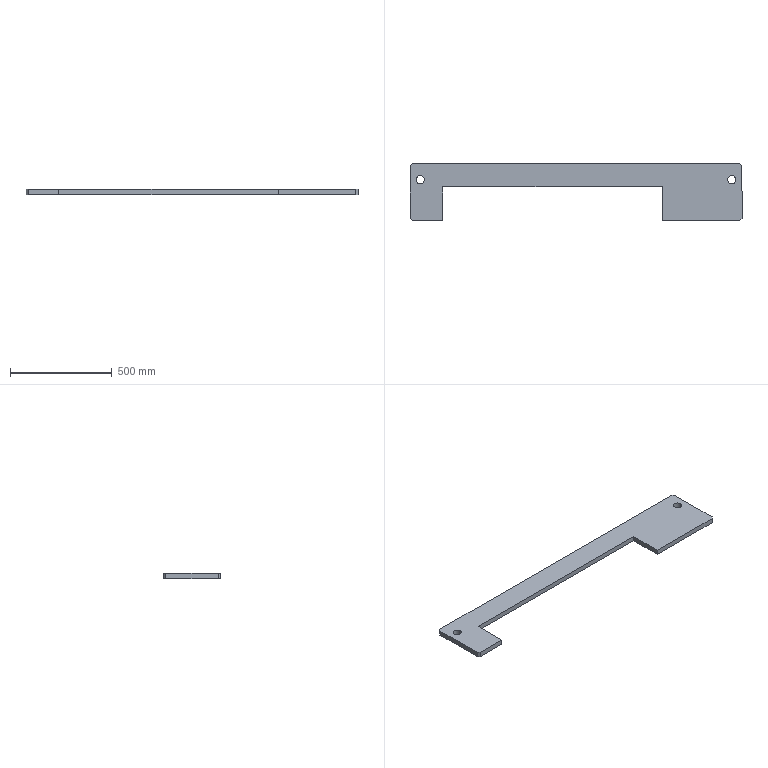Part | SolidWorks | features Chamfer 1, Extrusion 1, ICE 1 | 1 solid | 18 faces | box 1630 x 280 x 25 mm | volume 6887168 mm3 | plane 14 | cylinder 4 | commonest cylinder face diameters 40 x4
STEP:
#1=CARTESIAN_POINT('',(30.,-80.,0.));
#2=VERTEX_POINT('',#1);
#3=CARTESIAN_POINT('',(70.,-80.,0.));
#4=VERTEX_POINT('',#3);
#5=CARTESIAN_POINT('',(50.,-80.,0.));
#6=DIRECTION('',(0.,0.,1.));
#7=DIRECTION('',(1.,0.,0.));
#8=AXIS2_PLACEMENT_3D('',#5,#6,#7);
#9=CIRCLE('',#8,20.);
#10=EDGE_CURVE('',#2,#4,#9,.T.);
#11=ORIENTED_EDGE('',*,*,#10,.F.);
#12=CARTESIAN_POINT('',(30.,-80.,25.));
#13=VERTEX_POINT('',#12);
#14=CARTESIAN_POINT('',(30.,-80.,0.));
#15=DIRECTION('',(0.,0.,1.));
#16=VECTOR('',#15,1000.);
#17=LINE('',#14,#16);
#18=EDGE_CURVE('',#2,#13,#17,.T.);
#19=ORIENTED_EDGE('',*,*,#18,.T.);
#20=CARTESIAN_POINT('',(70.,-80.,25.));
#21=VERTEX_POINT('',#20);
#22=CARTESIAN_POINT('',(50.,-80.,25.));
#23=DIRECTION('',(0.,0.,1.));
#24=DIRECTION('',(1.,0.,0.));
#25=AXIS2_PLACEMENT_3D('',#22,#23,#24);
#26=CIRCLE('',#25,20.);
#27=EDGE_CURVE('',#13,#21,#26,.T.);
#28=ORIENTED_EDGE('',*,*,#27,.T.);
#29=CARTESIAN_POINT('',(70.,-80.,0.));
#30=DIRECTION('',(0.,0.,1.));
#31=VECTOR('',#30,1000.);
#32=LINE('',#29,#31);
#33=EDGE_CURVE('',#4,#21,#32,.T.);
#34=ORIENTED_EDGE('',*,*,#33,.F.);
#35=EDGE_LOOP('',(#11,#19,#28,#34));
#36=FACE_OUTER_BOUND('',#35,.T.);
#37=CARTESIAN_POINT('',(50.,-80.,0.));
#38=DIRECTION('',(0.,0.,1.));
#39=DIRECTION('',(1.,0.,0.));
#40=AXIS2_PLACEMENT_3D('',#37,#38,#39);
#41=CYLINDRICAL_SURFACE('',#40,20.);
#42=ADVANCED_FACE('',(#36),#41,.F.);
#43=CARTESIAN_POINT('',(1560.,-80.,0.));
#44=VERTEX_POINT('',#43);
#45=CARTESIAN_POINT('',(1600.,-80.,0.));
#46=VERTEX_POINT('',#45);
#47=CARTESIAN_POINT('',(1580.,-80.,0.));
#48=DIRECTION('',(0.,0.,1.));
#49=DIRECTION('',(1.,0.,0.));
#50=AXIS2_PLACEMENT_3D('',#47,#48,#49);
#51=CIRCLE('',#50,20.);
#52=EDGE_CURVE('',#44,#46,#51,.T.);
#53=ORIENTED_EDGE('',*,*,#52,.F.);
#54=CARTESIAN_POINT('',(1560.,-80.,25.));
#55=VERTEX_POINT('',#54);
#56=CARTESIAN_POINT('',(1560.,-80.,0.));
#57=DIRECTION('',(0.,0.,1.));
#58=VECTOR('',#57,1000.);
#59=LINE('',#56,#58);
#60=EDGE_CURVE('',#44,#55,#59,.T.);
#61=ORIENTED_EDGE('',*,*,#60,.T.);
#62=CARTESIAN_POINT('',(1600.,-80.,25.));
#63=VERTEX_POINT('',#62);
#64=CARTESIAN_POINT('',(1580.,-80.,25.));
#65=DIRECTION('',(0.,0.,1.));
#66=DIRECTION('',(1.,0.,0.));
#67=AXIS2_PLACEMENT_3D('',#64,#65,#66);
#68=CIRCLE('',#67,20.);
#69=EDGE_CURVE('',#55,#63,#68,.T.);
#70=ORIENTED_EDGE('',*,*,#69,.T.);
#71=CARTESIAN_POINT('',(1600.,-80.,0.));
#72=DIRECTION('',(0.,0.,1.));
#73=VECTOR('',#72,1000.);
#74=LINE('',#71,#73);
#75=EDGE_CURVE('',#46,#63,#74,.T.);
#76=ORIENTED_EDGE('',*,*,#75,.F.);
#77=EDGE_LOOP('',(#53,#61,#70,#76));
#78=FACE_OUTER_BOUND('',#77,.T.);
#79=CARTESIAN_POINT('',(1580.,-80.,0.));
#80=DIRECTION('',(0.,0.,1.));
#81=DIRECTION('',(1.,0.,0.));
#82=AXIS2_PLACEMENT_3D('',#79,#80,#81);
#83=CYLINDRICAL_SURFACE('',#82,20.);
#84=ADVANCED_FACE('',(#78),#83,.F.);
#85=CARTESIAN_POINT('',(1240.,-280.,0.));
#86=VERTEX_POINT('',#85);
#87=CARTESIAN_POINT('',(1620.,-280.,0.));
#88=VERTEX_POINT('',#87);
#89=CARTESIAN_POINT('',(1630.,-280.,0.));
#90=DIRECTION('',(1.,0.,0.));
#91=VECTOR('',#90,1000.);
#92=LINE('',#89,#91);
#93=EDGE_CURVE('',#86,#88,#92,.T.);
#94=ORIENTED_EDGE('',*,*,#93,.T.);
#95=CARTESIAN_POINT('',(1620.,-280.,25.));
#96=VERTEX_POINT('',#95);
#97=CARTESIAN_POINT('',(1620.,-280.,25.));
#98=DIRECTION('',(0.,0.,1.));
#99=VECTOR('',#98,1000.);
#100=LINE('',#97,#99);
#101=EDGE_CURVE('',#88,#96,#100,.T.);
#102=ORIENTED_EDGE('',*,*,#101,.T.);
#103=CARTESIAN_POINT('',(1240.,-280.,25.));
#104=VERTEX_POINT('',#103);
#105=CARTESIAN_POINT('',(1630.,-280.,25.));
#106=DIRECTION('',(1.,0.,0.));
#107=VECTOR('',#106,1000.);
#108=LINE('',#105,#107);
#109=EDGE_CURVE('',#104,#96,#108,.T.);
#110=ORIENTED_EDGE('',*,*,#109,.F.);
#111=CARTESIAN_POINT('',(1240.,-280.,25.));
#112=DIRECTION('',(0.,0.,-1.));
#113=VECTOR('',#112,1000.);
#114=LINE('',#111,#113);
#115=EDGE_CURVE('',#104,#86,#114,.T.);
#116=ORIENTED_EDGE('',*,*,#115,.T.);
#117=EDGE_LOOP('',(#94,#102,#110,#116));
#118=FACE_OUTER_BOUND('',#117,.T.);
#119=CARTESIAN_POINT('',(1630.,-280.,25.));
#120=DIRECTION('',(0.,1.,0.));
#121=DIRECTION('',(0.,0.,1.));
#122=AXIS2_PLACEMENT_3D('',#119,#120,#121);
#123=PLANE('',#122);
#124=ADVANCED_FACE('',(#118),#123,.F.);
#125=CARTESIAN_POINT('',(1630.,-270.,25.));
#126=VERTEX_POINT('',#125);
#127=CARTESIAN_POINT('',(1630.,-10.,25.));
#128=VERTEX_POINT('',#127);
#129=CARTESIAN_POINT('',(1630.,0.,25.));
#130=DIRECTION('',(0.,1.,0.));
#131=VECTOR('',#130,1000.);
#132=LINE('',#129,#131);
#133=EDGE_CURVE('',#126,#128,#132,.T.);
#134=ORIENTED_EDGE('',*,*,#133,.F.);
#135=CARTESIAN_POINT('',(1630.,-270.,0.));
#136=VERTEX_POINT('',#135);
#137=CARTESIAN_POINT('',(1630.,-270.,25.));
#138=DIRECTION('',(0.,0.,-1.));
#139=VECTOR('',#138,1000.);
#140=LINE('',#137,#139);
#141=EDGE_CURVE('',#126,#136,#140,.T.);
#142=ORIENTED_EDGE('',*,*,#141,.T.);
#143=CARTESIAN_POINT('',(1630.,-10.,0.));
#144=VERTEX_POINT('',#143);
#145=CARTESIAN_POINT('',(1630.,0.,0.));
#146=DIRECTION('',(0.,1.,0.));
#147=VECTOR('',#146,1000.);
#148=LINE('',#145,#147);
#149=EDGE_CURVE('',#136,#144,#148,.T.);
#150=ORIENTED_EDGE('',*,*,#149,.T.);
#151=CARTESIAN_POINT('',(1630.,-10.,25.));
#152=DIRECTION('',(0.,0.,1.));
#153=VECTOR('',#152,1000.);
#154=LINE('',#151,#153);
#155=EDGE_CURVE('',#144,#128,#154,.T.);
#156=ORIENTED_EDGE('',*,*,#155,.T.);
#157=EDGE_LOOP('',(#134,#142,#150,#156));
#158=FACE_OUTER_BOUND('',#157,.T.);
#159=CARTESIAN_POINT('',(1630.,0.,25.));
#160=DIRECTION('',(-1.,0.,0.));
#161=DIRECTION('',(0.,-1.,0.));
#162=AXIS2_PLACEMENT_3D('',#159,#160,#161);
#163=PLANE('',#162);
#164=ADVANCED_FACE('',(#158),#163,.F.);
#165=CARTESIAN_POINT('',(1620.,0.,0.));
#166=VERTEX_POINT('',#165);
#167=CARTESIAN_POINT('',(10.,0.,0.));
#168=VERTEX_POINT('',#167);
#169=CARTESIAN_POINT('',(1630.,0.,0.));
#170=DIRECTION('',(-1.,0.,0.));
#171=VECTOR('',#170,1000.);
#172=LINE('',#169,#171);
#173=EDGE_CURVE('',#166,#168,#172,.T.);
#174=ORIENTED_EDGE('',*,*,#173,.T.);
#175=CARTESIAN_POINT('',(10.,0.,25.));
#176=VERTEX_POINT('',#175);
#177=CARTESIAN_POINT('',(10.,0.,25.));
#178=DIRECTION('',(0.,0.,1.));
#179=VECTOR('',#178,1000.);
#180=LINE('',#177,#179);
#181=EDGE_CURVE('',#168,#176,#180,.T.);
#182=ORIENTED_EDGE('',*,*,#181,.T.);
#183=CARTESIAN_POINT('',(1620.,0.,25.));
#184=VERTEX_POINT('',#183);
#185=CARTESIAN_POINT('',(1630.,0.,25.));
#186=DIRECTION('',(-1.,0.,0.));
#187=VECTOR('',#186,1000.);
#188=LINE('',#185,#187);
#189=EDGE_CURVE('',#184,#176,#188,.T.);
#190=ORIENTED_EDGE('',*,*,#189,.F.);
#191=CARTESIAN_POINT('',(1620.,0.,25.));
#192=DIRECTION('',(0.,0.,-1.));
#193=VECTOR('',#192,1000.);
#194=LINE('',#191,#193);
#195=EDGE_CURVE('',#184,#166,#194,.T.);
#196=ORIENTED_EDGE('',*,*,#195,.T.);
#197=EDGE_LOOP('',(#174,#182,#190,#196));
#198=FACE_OUTER_BOUND('',#197,.T.);
#199=CARTESIAN_POINT('',(1630.,0.,25.));
#200=DIRECTION('',(0.,-1.,0.));
#201=DIRECTION('',(1.,0.,0.));
#202=AXIS2_PLACEMENT_3D('',#199,#200,#201);
#203=PLANE('',#202);
#204=ADVANCED_FACE('',(#198),#203,.F.);
#205=CARTESIAN_POINT('',(0.,-10.,25.));
#206=VERTEX_POINT('',#205);
#207=CARTESIAN_POINT('',(0.,-270.,25.));
#208=VERTEX_POINT('',#207);
#209=CARTESIAN_POINT('',(0.,0.,25.));
#210=DIRECTION('',(0.,-1.,0.));
#211=VECTOR('',#210,1000.);
#212=LINE('',#209,#211);
#213=EDGE_CURVE('',#206,#208,#212,.T.);
#214=ORIENTED_EDGE('',*,*,#213,.F.);
#215=CARTESIAN_POINT('',(0.,-10.,0.));
#216=VERTEX_POINT('',#215);
#217=CARTESIAN_POINT('',(0.,-10.,25.));
#218=DIRECTION('',(0.,0.,-1.));
#219=VECTOR('',#218,1000.);
#220=LINE('',#217,#219);
#221=EDGE_CURVE('',#206,#216,#220,.T.);
#222=ORIENTED_EDGE('',*,*,#221,.T.);
#223=CARTESIAN_POINT('',(0.,-270.,0.));
#224=VERTEX_POINT('',#223);
#225=CARTESIAN_POINT('',(0.,0.,0.));
#226=DIRECTION('',(0.,-1.,0.));
#227=VECTOR('',#226,1000.);
#228=LINE('',#225,#227);
#229=EDGE_CURVE('',#216,#224,#228,.T.);
#230=ORIENTED_EDGE('',*,*,#229,.T.);
#231=CARTESIAN_POINT('',(0.,-270.,25.));
#232=DIRECTION('',(0.,0.,1.));
#233=VECTOR('',#232,1000.);
#234=LINE('',#231,#233);
#235=EDGE_CURVE('',#224,#208,#234,.T.);
#236=ORIENTED_EDGE('',*,*,#235,.T.);
#237=EDGE_LOOP('',(#214,#222,#230,#236));
#238=FACE_OUTER_BOUND('',#237,.T.);
#239=CARTESIAN_POINT('',(0.,0.,25.));
#240=DIRECTION('',(1.,0.,0.));
#241=DIRECTION('',(0.,1.,0.));
#242=AXIS2_PLACEMENT_3D('',#239,#240,#241);
#243=PLANE('',#242);
#244=ADVANCED_FACE('',(#238),#243,.F.);
#245=CARTESIAN_POINT('',(10.,-280.,25.));
#246=VERTEX_POINT('',#245);
#247=CARTESIAN_POINT('',(160.,-280.,25.));
#248=VERTEX_POINT('',#247);
#249=CARTESIAN_POINT('',(160.,-280.,25.));
#250=DIRECTION('',(1.,0.,0.));
#251=VECTOR('',#250,1000.);
#252=LINE('',#249,#251);
#253=EDGE_CURVE('',#246,#248,#252,.T.);
#254=ORIENTED_EDGE('',*,*,#253,.F.);
#255=CARTESIAN_POINT('',(10.,-280.,0.));
#256=VERTEX_POINT('',#255);
#257=CARTESIAN_POINT('',(10.,-280.,25.));
#258=DIRECTION('',(0.,0.,-1.));
#259=VECTOR('',#258,1000.);
#260=LINE('',#257,#259);
#261=EDGE_CURVE('',#246,#256,#260,.T.);
#262=ORIENTED_EDGE('',*,*,#261,.T.);
#263=CARTESIAN_POINT('',(160.,-280.,0.));
#264=VERTEX_POINT('',#263);
#265=CARTESIAN_POINT('',(160.,-280.,0.));
#266=DIRECTION('',(1.,0.,0.));
#267=VECTOR('',#266,1000.);
#268=LINE('',#265,#267);
#269=EDGE_CURVE('',#256,#264,#268,.T.);
#270=ORIENTED_EDGE('',*,*,#269,.T.);
#271=CARTESIAN_POINT('',(160.,-280.,25.));
#272=DIRECTION('',(0.,0.,-1.));
#273=VECTOR('',#272,1000.);
#274=LINE('',#271,#273);
#275=EDGE_CURVE('',#248,#264,#274,.T.);
#276=ORIENTED_EDGE('',*,*,#275,.F.);
#277=EDGE_LOOP('',(#254,#262,#270,#276));
#278=FACE_OUTER_BOUND('',#277,.T.);
#279=CARTESIAN_POINT('',(160.,-280.,25.));
#280=DIRECTION('',(0.,1.,0.));
#281=DIRECTION('',(0.,0.,1.));
#282=AXIS2_PLACEMENT_3D('',#279,#280,#281);
#283=PLANE('',#282);
#284=ADVANCED_FACE('',(#278),#283,.F.);
#285=CARTESIAN_POINT('',(160.,-115.,0.));
#286=VERTEX_POINT('',#285);
#287=CARTESIAN_POINT('',(160.,-115.,0.));
#288=DIRECTION('',(0.,1.,0.));
#289=VECTOR('',#288,1000.);
#290=LINE('',#287,#289);
#291=EDGE_CURVE('',#264,#286,#290,.T.);
#292=ORIENTED_EDGE('',*,*,#291,.T.);
#293=CARTESIAN_POINT('',(160.,-115.,25.));
#294=VERTEX_POINT('',#293);
#295=CARTESIAN_POINT('',(160.,-115.,25.));
#296=DIRECTION('',(0.,0.,-1.));
#297=VECTOR('',#296,1000.);
#298=LINE('',#295,#297);
#299=EDGE_CURVE('',#294,#286,#298,.T.);
#300=ORIENTED_EDGE('',*,*,#299,.F.);
#301=CARTESIAN_POINT('',(160.,-115.,25.));
#302=DIRECTION('',(0.,1.,0.));
#303=VECTOR('',#302,1000.);
#304=LINE('',#301,#303);
#305=EDGE_CURVE('',#248,#294,#304,.T.);
#306=ORIENTED_EDGE('',*,*,#305,.F.);
#307=ORIENTED_EDGE('',*,*,#275,.T.);
#308=EDGE_LOOP('',(#292,#300,#306,#307));
#309=FACE_OUTER_BOUND('',#308,.T.);
#310=CARTESIAN_POINT('',(160.,-115.,25.));
#311=DIRECTION('',(-1.,0.,0.));
#312=DIRECTION('',(0.,-1.,0.));
#313=AXIS2_PLACEMENT_3D('',#310,#311,#312);
#314=PLANE('',#313);
#315=ADVANCED_FACE('',(#309),#314,.F.);
#316=CARTESIAN_POINT('',(1240.,-115.,0.));
#317=VERTEX_POINT('',#316);
#318=CARTESIAN_POINT('',(160.,-115.,0.));
#319=DIRECTION('',(1.,0.,0.));
#320=VECTOR('',#319,1000.);
#321=LINE('',#318,#320);
#322=EDGE_CURVE('',#286,#317,#321,.T.);
#323=ORIENTED_EDGE('',*,*,#322,.T.);
#324=CARTESIAN_POINT('',(1240.,-115.,25.));
#325=VERTEX_POINT('',#324);
#326=CARTESIAN_POINT('',(1240.,-115.,25.));
#327=DIRECTION('',(0.,0.,-1.));
#328=VECTOR('',#327,1000.);
#329=LINE('',#326,#328);
#330=EDGE_CURVE('',#325,#317,#329,.T.);
#331=ORIENTED_EDGE('',*,*,#330,.F.);
#332=CARTESIAN_POINT('',(160.,-115.,25.));
#333=DIRECTION('',(1.,0.,0.));
#334=VECTOR('',#333,1000.);
#335=LINE('',#332,#334);
#336=EDGE_CURVE('',#294,#325,#335,.T.);
#337=ORIENTED_EDGE('',*,*,#336,.F.);
#338=ORIENTED_EDGE('',*,*,#299,.T.);
#339=EDGE_LOOP('',(#323,#331,#337,#338));
#340=FACE_OUTER_BOUND('',#339,.T.);
#341=CARTESIAN_POINT('',(160.,-115.,25.));
#342=DIRECTION('',(0.,1.,0.));
#343=DIRECTION('',(0.,0.,1.));
#344=AXIS2_PLACEMENT_3D('',#341,#342,#343);
#345=PLANE('',#344);
#346=ADVANCED_FACE('',(#340),#345,.F.);
#347=CARTESIAN_POINT('',(1240.,-115.,0.));
#348=DIRECTION('',(0.,-1.,0.));
#349=VECTOR('',#348,1000.);
#350=LINE('',#347,#349);
#351=EDGE_CURVE('',#317,#86,#350,.T.);
#352=ORIENTED_EDGE('',*,*,#351,.T.);
#353=ORIENTED_EDGE('',*,*,#115,.F.);
#354=CARTESIAN_POINT('',(1240.,-115.,25.));
#355=DIRECTION('',(0.,-1.,0.));
#356=VECTOR('',#355,1000.);
#357=LINE('',#354,#356);
#358=EDGE_CURVE('',#325,#104,#357,.T.);
#359=ORIENTED_EDGE('',*,*,#358,.F.);
#360=ORIENTED_EDGE('',*,*,#330,.T.);
#361=EDGE_LOOP('',(#352,#353,#359,#360));
#362=FACE_OUTER_BOUND('',#361,.T.);
#363=CARTESIAN_POINT('',(1240.,-115.,25.));
#364=DIRECTION('',(1.,0.,0.));
#365=DIRECTION('',(0.,0.,-1.));
#366=AXIS2_PLACEMENT_3D('',#363,#364,#365);
#367=PLANE('',#366);
#368=ADVANCED_FACE('',(#362),#367,.F.);
#369=CARTESIAN_POINT('',(50.,-80.,25.));
#370=DIRECTION('',(0.,0.,1.));
#371=DIRECTION('',(1.,0.,0.));
#372=AXIS2_PLACEMENT_3D('',#369,#370,#371);
#373=CIRCLE('',#372,20.);
#374=EDGE_CURVE('',#21,#13,#373,.T.);
#375=ORIENTED_EDGE('',*,*,#374,.F.);
#376=ORIENTED_EDGE('',*,*,#27,.F.);
#377=EDGE_LOOP('',(#375,#376));
#378=FACE_BOUND('',#377,.T.);
#379=CARTESIAN_POINT('',(1580.,-80.,25.));
#380=DIRECTION('',(0.,0.,1.));
#381=DIRECTION('',(1.,0.,0.));
#382=AXIS2_PLACEMENT_3D('',#379,#380,#381);
#383=CIRCLE('',#382,20.);
#384=EDGE_CURVE('',#63,#55,#383,.T.);
#385=ORIENTED_EDGE('',*,*,#384,.F.);
#386=ORIENTED_EDGE('',*,*,#69,.F.);
#387=EDGE_LOOP('',(#385,#386));
#388=FACE_BOUND('',#387,.T.);
#389=ORIENTED_EDGE('',*,*,#189,.T.);
#390=CARTESIAN_POINT('',(5.,-5.,25.));
#391=DIRECTION('',(-0.7071,-0.7071,0.));
#392=VECTOR('',#391,1000.);
#393=LINE('',#390,#392);
#394=EDGE_CURVE('',#176,#206,#393,.T.);
#395=ORIENTED_EDGE('',*,*,#394,.T.);
#396=ORIENTED_EDGE('',*,*,#213,.T.);
#397=CARTESIAN_POINT('',(-135.,-135.,25.));
#398=DIRECTION('',(0.7071,-0.7071,0.));
#399=VECTOR('',#398,1000.);
#400=LINE('',#397,#399);
#401=EDGE_CURVE('',#208,#246,#400,.T.);
#402=ORIENTED_EDGE('',*,*,#401,.T.);
#403=ORIENTED_EDGE('',*,*,#253,.T.);
#404=ORIENTED_EDGE('',*,*,#305,.T.);
#405=ORIENTED_EDGE('',*,*,#336,.T.);
#406=ORIENTED_EDGE('',*,*,#358,.T.);
#407=ORIENTED_EDGE('',*,*,#109,.T.);
#408=CARTESIAN_POINT('',(950.,-950.,25.));
#409=DIRECTION('',(0.7071,0.7071,0.));
#410=VECTOR('',#409,1000.);
#411=LINE('',#408,#410);
#412=EDGE_CURVE('',#96,#126,#411,.T.);
#413=ORIENTED_EDGE('',*,*,#412,.T.);
#414=ORIENTED_EDGE('',*,*,#133,.T.);
#415=CARTESIAN_POINT('',(810.,810.,25.));
#416=DIRECTION('',(-0.7071,0.7071,0.));
#417=VECTOR('',#416,1000.);
#418=LINE('',#415,#417);
#419=EDGE_CURVE('',#128,#184,#418,.T.);
#420=ORIENTED_EDGE('',*,*,#419,.T.);
#421=EDGE_LOOP('',(#389,#395,#396,#402,#403,#404,#405,#406,#407,#413,#414,#420));
#422=FACE_OUTER_BOUND('',#421,.T.);
#423=CARTESIAN_POINT('',(0.,0.,25.));
#424=DIRECTION('',(0.,0.,1.));
#425=DIRECTION('',(1.,0.,0.));
#426=AXIS2_PLACEMENT_3D('',#423,#424,#425);
#427=PLANE('',#426);
#428=ADVANCED_FACE('',(#378,#388,#422),#427,.T.);
#429=CARTESIAN_POINT('',(50.,-80.,0.));
#430=DIRECTION('',(0.,0.,1.));
#431=DIRECTION('',(1.,0.,0.));
#432=AXIS2_PLACEMENT_3D('',#429,#430,#431);
#433=CIRCLE('',#432,20.);
#434=EDGE_CURVE('',#4,#2,#433,.T.);
#435=ORIENTED_EDGE('',*,*,#434,.T.);
#436=ORIENTED_EDGE('',*,*,#10,.T.);
#437=EDGE_LOOP('',(#435,#436));
#438=FACE_BOUND('',#437,.T.);
#439=CARTESIAN_POINT('',(1580.,-80.,0.));
#440=DIRECTION('',(0.,0.,1.));
#441=DIRECTION('',(1.,0.,0.));
#442=AXIS2_PLACEMENT_3D('',#439,#440,#441);
#443=CIRCLE('',#442,20.);
#444=EDGE_CURVE('',#46,#44,#443,.T.);
#445=ORIENTED_EDGE('',*,*,#444,.T.);
#446=ORIENTED_EDGE('',*,*,#52,.T.);
#447=EDGE_LOOP('',(#445,#446));
#448=FACE_BOUND('',#447,.T.);
#449=ORIENTED_EDGE('',*,*,#229,.F.);
#450=CARTESIAN_POINT('',(0.,-10.,0.));
#451=DIRECTION('',(0.7071,0.7071,0.));
#452=VECTOR('',#451,1000.);
#453=LINE('',#450,#452);
#454=EDGE_CURVE('',#216,#168,#453,.T.);
#455=ORIENTED_EDGE('',*,*,#454,.T.);
#456=ORIENTED_EDGE('',*,*,#173,.F.);
#457=CARTESIAN_POINT('',(1620.,0.,0.));
#458=DIRECTION('',(0.7071,-0.7071,0.));
#459=VECTOR('',#458,1000.);
#460=LINE('',#457,#459);
#461=EDGE_CURVE('',#166,#144,#460,.T.);
#462=ORIENTED_EDGE('',*,*,#461,.T.);
#463=ORIENTED_EDGE('',*,*,#149,.F.);
#464=CARTESIAN_POINT('',(1630.,-270.,0.));
#465=DIRECTION('',(-0.7071,-0.7071,0.));
#466=VECTOR('',#465,1000.);
#467=LINE('',#464,#466);
#468=EDGE_CURVE('',#136,#88,#467,.T.);
#469=ORIENTED_EDGE('',*,*,#468,.T.);
#470=ORIENTED_EDGE('',*,*,#93,.F.);
#471=ORIENTED_EDGE('',*,*,#351,.F.);
#472=ORIENTED_EDGE('',*,*,#322,.F.);
#473=ORIENTED_EDGE('',*,*,#291,.F.);
#474=ORIENTED_EDGE('',*,*,#269,.F.);
#475=CARTESIAN_POINT('',(10.,-280.,0.));
#476=DIRECTION('',(-0.7071,0.7071,0.));
#477=VECTOR('',#476,1000.);
#478=LINE('',#475,#477);
#479=EDGE_CURVE('',#256,#224,#478,.T.);
#480=ORIENTED_EDGE('',*,*,#479,.T.);
#481=EDGE_LOOP('',(#449,#455,#456,#462,#463,#469,#470,#471,#472,#473,#474,#480));
#482=FACE_OUTER_BOUND('',#481,.T.);
#483=CARTESIAN_POINT('',(0.,0.,0.));
#484=DIRECTION('',(0.,0.,1.));
#485=DIRECTION('',(1.,0.,0.));
#486=AXIS2_PLACEMENT_3D('',#483,#484,#485);
#487=PLANE('',#486);
#488=ADVANCED_FACE('',(#438,#448,#482),#487,.F.);
#489=ORIENTED_EDGE('',*,*,#394,.F.);
#490=ORIENTED_EDGE('',*,*,#181,.F.);
#491=ORIENTED_EDGE('',*,*,#454,.F.);
#492=ORIENTED_EDGE('',*,*,#221,.F.);
#493=EDGE_LOOP('',(#489,#490,#491,#492));
#494=FACE_OUTER_BOUND('',#493,.T.);
#495=CARTESIAN_POINT('',(0.,-10.,25.));
#496=DIRECTION('',(0.7071,-0.7071,0.));
#497=DIRECTION('',(0.,0.,-1.));
#498=AXIS2_PLACEMENT_3D('',#495,#496,#497);
#499=PLANE('',#498);
#500=ADVANCED_FACE('',(#494),#499,.F.);
#501=ORIENTED_EDGE('',*,*,#401,.F.);
#502=ORIENTED_EDGE('',*,*,#235,.F.);
#503=ORIENTED_EDGE('',*,*,#479,.F.);
#504=ORIENTED_EDGE('',*,*,#261,.F.);
#505=EDGE_LOOP('',(#501,#502,#503,#504));
#506=FACE_OUTER_BOUND('',#505,.T.);
#507=CARTESIAN_POINT('',(10.,-280.,25.));
#508=DIRECTION('',(0.7071,0.7071,0.));
#509=DIRECTION('',(0.,0.,-1.));
#510=AXIS2_PLACEMENT_3D('',#507,#508,#509);
#511=PLANE('',#510);
#512=ADVANCED_FACE('',(#506),#511,.F.);
#513=ORIENTED_EDGE('',*,*,#412,.F.);
#514=ORIENTED_EDGE('',*,*,#101,.F.);
#515=ORIENTED_EDGE('',*,*,#468,.F.);
#516=ORIENTED_EDGE('',*,*,#141,.F.);
#517=EDGE_LOOP('',(#513,#514,#515,#516));
#518=FACE_OUTER_BOUND('',#517,.T.);
#519=CARTESIAN_POINT('',(1630.,-270.,25.));
#520=DIRECTION('',(-0.7071,0.7071,0.));
#521=DIRECTION('',(0.,0.,-1.));
#522=AXIS2_PLACEMENT_3D('',#519,#520,#521);
#523=PLANE('',#522);
#524=ADVANCED_FACE('',(#518),#523,.F.);
#525=ORIENTED_EDGE('',*,*,#419,.F.);
#526=ORIENTED_EDGE('',*,*,#155,.F.);
#527=ORIENTED_EDGE('',*,*,#461,.F.);
#528=ORIENTED_EDGE('',*,*,#195,.F.);
#529=EDGE_LOOP('',(#525,#526,#527,#528));
#530=FACE_OUTER_BOUND('',#529,.T.);
#531=CARTESIAN_POINT('',(1620.,0.,25.));
#532=DIRECTION('',(-0.7071,-0.7071,0.));
#533=DIRECTION('',(0.,0.,-1.));
#534=AXIS2_PLACEMENT_3D('',#531,#532,#533);
#535=PLANE('',#534);
#536=ADVANCED_FACE('',(#530),#535,.F.);
#537=ORIENTED_EDGE('',*,*,#60,.F.);
#538=ORIENTED_EDGE('',*,*,#444,.F.);
#539=ORIENTED_EDGE('',*,*,#75,.T.);
#540=ORIENTED_EDGE('',*,*,#384,.T.);
#541=EDGE_LOOP('',(#537,#538,#539,#540));
#542=FACE_OUTER_BOUND('',#541,.T.);
#543=CARTESIAN_POINT('',(1580.,-80.,0.));
#544=DIRECTION('',(0.,0.,1.));
#545=DIRECTION('',(1.,0.,0.));
#546=AXIS2_PLACEMENT_3D('',#543,#544,#545);
#547=CYLINDRICAL_SURFACE('',#546,20.);
#548=ADVANCED_FACE('',(#542),#547,.F.);
#549=ORIENTED_EDGE('',*,*,#18,.F.);
#550=ORIENTED_EDGE('',*,*,#434,.F.);
#551=ORIENTED_EDGE('',*,*,#33,.T.);
#552=ORIENTED_EDGE('',*,*,#374,.T.);
#553=EDGE_LOOP('',(#549,#550,#551,#552));
#554=FACE_OUTER_BOUND('',#553,.T.);
#555=CARTESIAN_POINT('',(50.,-80.,0.));
#556=DIRECTION('',(0.,0.,1.));
#557=DIRECTION('',(1.,0.,0.));
#558=AXIS2_PLACEMENT_3D('',#555,#556,#557);
#559=CYLINDRICAL_SURFACE('',#558,20.);
#560=ADVANCED_FACE('',(#554),#559,.F.);
#561=CLOSED_SHELL('',(#42,#84,#124,#164,#204,#244,#284,#315,#346,#368,#428,#488,#500,#512,#524,#536,#548,#560));
#562=MANIFOLD_SOLID_BREP('',#561);
#563=CARTESIAN_POINT('',(0.,0.,0.));
#564=DIRECTION('',(0.,0.,1.));
#565=DIRECTION('',(1.,0.,0.));
#566=AXIS2_PLACEMENT_3D('',#563,#564,#565);
#567=(LENGTH_UNIT()NAMED_UNIT(*)SI_UNIT(.MILLI.,.METRE.));
#568=UNCERTAINTY_MEASURE_WITH_UNIT(LENGTH_MEASURE(0.00001),#567,'','');
#569=(NAMED_UNIT(*)PLANE_ANGLE_UNIT()SI_UNIT($,.RADIAN.));
#570=(NAMED_UNIT(*)SI_UNIT($,.STERADIAN.)SOLID_ANGLE_UNIT());
#571=(GEOMETRIC_REPRESENTATION_CONTEXT(3)GLOBAL_UNCERTAINTY_ASSIGNED_CONTEXT((#568))GLOBAL_UNIT_ASSIGNED_CONTEXT((#567,#569,#570))REPRESENTATION_CONTEXT('',''));
#572=ADVANCED_BREP_SHAPE_REPRESENTATION('',(#562,#566),#571);